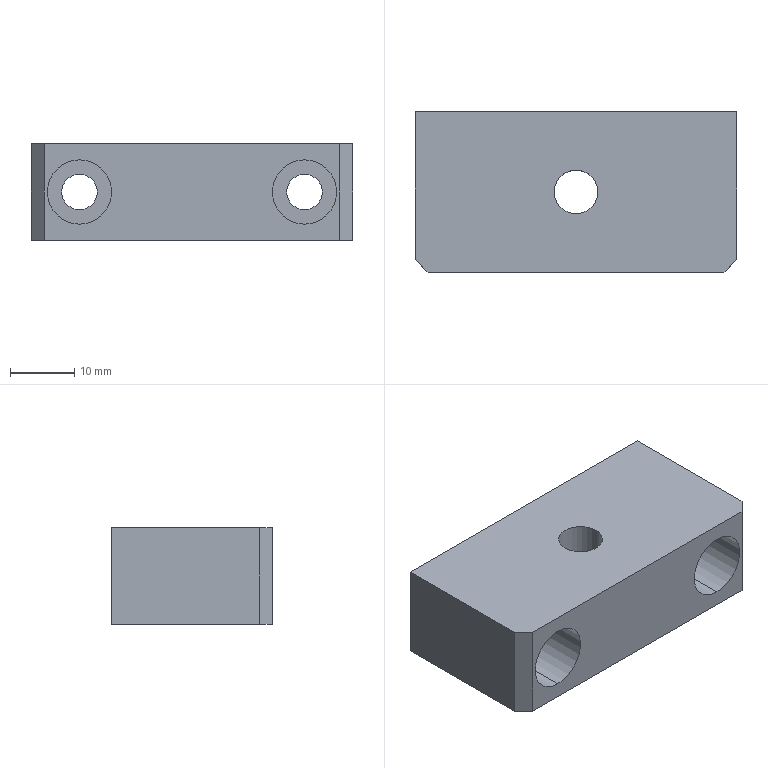Part | SolidWorks | features HoleWzd 2, Chamfer 1, Extrusion 1 | 1 solid | 20 faces | box 50 x 25 x 15 mm | volume 15237 mm3 | cylinder 10 | plane 10 | commonest cylinder face diameters 5.5 x4 10 x4 6.8 x2
STEP:
#1=CARTESIAN_POINT('',(-3.4,0.,0.));
#2=VERTEX_POINT('',#1);
#3=CARTESIAN_POINT('',(3.4,0.,0.));
#4=VERTEX_POINT('',#3);
#5=CARTESIAN_POINT('',(0.,0.,0.));
#6=DIRECTION('',(0.,0.,1.));
#7=DIRECTION('',(1.,0.,0.));
#8=AXIS2_PLACEMENT_3D('',#5,#6,#7);
#9=CIRCLE('',#8,3.4);
#10=EDGE_CURVE('',#2,#4,#9,.T.);
#11=ORIENTED_EDGE('',*,*,#10,.F.);
#12=CARTESIAN_POINT('',(-3.4,0.,15.));
#13=VERTEX_POINT('',#12);
#14=CARTESIAN_POINT('',(-3.4,0.,15.));
#15=DIRECTION('',(0.,0.,1.));
#16=VECTOR('',#15,1000.);
#17=LINE('',#14,#16);
#18=EDGE_CURVE('',#2,#13,#17,.T.);
#19=ORIENTED_EDGE('',*,*,#18,.T.);
#20=CARTESIAN_POINT('',(3.4,0.,15.));
#21=VERTEX_POINT('',#20);
#22=CARTESIAN_POINT('',(0.,0.,15.));
#23=DIRECTION('',(0.,0.,1.));
#24=DIRECTION('',(1.,0.,0.));
#25=AXIS2_PLACEMENT_3D('',#22,#23,#24);
#26=CIRCLE('',#25,3.4);
#27=EDGE_CURVE('',#13,#21,#26,.T.);
#28=ORIENTED_EDGE('',*,*,#27,.T.);
#29=CARTESIAN_POINT('',(3.4,0.,15.));
#30=DIRECTION('',(0.,0.,1.));
#31=VECTOR('',#30,1000.);
#32=LINE('',#29,#31);
#33=EDGE_CURVE('',#4,#21,#32,.T.);
#34=ORIENTED_EDGE('',*,*,#33,.F.);
#35=EDGE_LOOP('',(#11,#19,#28,#34));
#36=FACE_OUTER_BOUND('',#35,.T.);
#37=CARTESIAN_POINT('',(0.,0.,15.));
#38=DIRECTION('',(0.,0.,1.));
#39=DIRECTION('',(1.,0.,0.));
#40=AXIS2_PLACEMENT_3D('',#37,#38,#39);
#41=CYLINDRICAL_SURFACE('',#40,3.4);
#42=ADVANCED_FACE('',(#36),#41,.F.);
#43=CARTESIAN_POINT('',(17.5,3.2,12.5));
#44=VERTEX_POINT('',#43);
#45=CARTESIAN_POINT('',(17.5,3.2,2.5));
#46=VERTEX_POINT('',#45);
#47=CARTESIAN_POINT('',(17.5,3.2,7.5));
#48=DIRECTION('',(0.,-1.,0.));
#49=DIRECTION('',(0.,0.,-1.));
#50=AXIS2_PLACEMENT_3D('',#47,#48,#49);
#51=CIRCLE('',#50,5.);
#52=EDGE_CURVE('',#44,#46,#51,.T.);
#53=ORIENTED_EDGE('',*,*,#52,.F.);
#54=CARTESIAN_POINT('',(17.5,-12.5,12.5));
#55=VERTEX_POINT('',#54);
#56=CARTESIAN_POINT('',(17.5,-12.5,12.5));
#57=DIRECTION('',(0.,-1.,0.));
#58=VECTOR('',#57,1000.);
#59=LINE('',#56,#58);
#60=EDGE_CURVE('',#44,#55,#59,.T.);
#61=ORIENTED_EDGE('',*,*,#60,.T.);
#62=CARTESIAN_POINT('',(17.5,-12.5,2.5));
#63=VERTEX_POINT('',#62);
#64=CARTESIAN_POINT('',(17.5,-12.5,7.5));
#65=DIRECTION('',(0.,-1.,0.));
#66=DIRECTION('',(0.,0.,-1.));
#67=AXIS2_PLACEMENT_3D('',#64,#65,#66);
#68=CIRCLE('',#67,5.);
#69=EDGE_CURVE('',#55,#63,#68,.T.);
#70=ORIENTED_EDGE('',*,*,#69,.T.);
#71=CARTESIAN_POINT('',(17.5,-12.5,2.5));
#72=DIRECTION('',(0.,-1.,0.));
#73=VECTOR('',#72,1000.);
#74=LINE('',#71,#73);
#75=EDGE_CURVE('',#46,#63,#74,.T.);
#76=ORIENTED_EDGE('',*,*,#75,.F.);
#77=EDGE_LOOP('',(#53,#61,#70,#76));
#78=FACE_OUTER_BOUND('',#77,.T.);
#79=CARTESIAN_POINT('',(17.5,-12.5,7.5));
#80=DIRECTION('',(0.,-1.,0.));
#81=DIRECTION('',(0.,0.,-1.));
#82=AXIS2_PLACEMENT_3D('',#79,#80,#81);
#83=CYLINDRICAL_SURFACE('',#82,5.);
#84=ADVANCED_FACE('',(#78),#83,.F.);
#85=CARTESIAN_POINT('',(17.5,12.5,10.25));
#86=VERTEX_POINT('',#85);
#87=CARTESIAN_POINT('',(17.5,12.5,4.75));
#88=VERTEX_POINT('',#87);
#89=CARTESIAN_POINT('',(17.5,12.5,7.5));
#90=DIRECTION('',(0.,-1.,0.));
#91=DIRECTION('',(0.,0.,-1.));
#92=AXIS2_PLACEMENT_3D('',#89,#90,#91);
#93=CIRCLE('',#92,2.75);
#94=EDGE_CURVE('',#86,#88,#93,.T.);
#95=ORIENTED_EDGE('',*,*,#94,.F.);
#96=CARTESIAN_POINT('',(17.5,3.2,10.25));
#97=VERTEX_POINT('',#96);
#98=CARTESIAN_POINT('',(17.5,-12.5,10.25));
#99=DIRECTION('',(0.,-1.,0.));
#100=VECTOR('',#99,1000.);
#101=LINE('',#98,#100);
#102=EDGE_CURVE('',#86,#97,#101,.T.);
#103=ORIENTED_EDGE('',*,*,#102,.T.);
#104=CARTESIAN_POINT('',(17.5,3.2,4.75));
#105=VERTEX_POINT('',#104);
#106=CARTESIAN_POINT('',(17.5,3.2,7.5));
#107=DIRECTION('',(0.,-1.,0.));
#108=DIRECTION('',(0.,0.,-1.));
#109=AXIS2_PLACEMENT_3D('',#106,#107,#108);
#110=CIRCLE('',#109,2.75);
#111=EDGE_CURVE('',#97,#105,#110,.T.);
#112=ORIENTED_EDGE('',*,*,#111,.T.);
#113=CARTESIAN_POINT('',(17.5,-12.5,4.75));
#114=DIRECTION('',(0.,-1.,0.));
#115=VECTOR('',#114,1000.);
#116=LINE('',#113,#115);
#117=EDGE_CURVE('',#88,#105,#116,.T.);
#118=ORIENTED_EDGE('',*,*,#117,.F.);
#119=EDGE_LOOP('',(#95,#103,#112,#118));
#120=FACE_OUTER_BOUND('',#119,.T.);
#121=CARTESIAN_POINT('',(17.5,-12.5,7.5));
#122=DIRECTION('',(0.,-1.,0.));
#123=DIRECTION('',(0.,0.,-1.));
#124=AXIS2_PLACEMENT_3D('',#121,#122,#123);
#125=CYLINDRICAL_SURFACE('',#124,2.75);
#126=ADVANCED_FACE('',(#120),#125,.F.);
#127=CARTESIAN_POINT('',(-17.5,3.2,12.5));
#128=VERTEX_POINT('',#127);
#129=CARTESIAN_POINT('',(-17.5,3.2,2.5));
#130=VERTEX_POINT('',#129);
#131=CARTESIAN_POINT('',(-17.5,3.2,7.5));
#132=DIRECTION('',(0.,-1.,0.));
#133=DIRECTION('',(0.,0.,-1.));
#134=AXIS2_PLACEMENT_3D('',#131,#132,#133);
#135=CIRCLE('',#134,5.);
#136=EDGE_CURVE('',#128,#130,#135,.T.);
#137=ORIENTED_EDGE('',*,*,#136,.F.);
#138=CARTESIAN_POINT('',(-17.5,-12.5,12.5));
#139=VERTEX_POINT('',#138);
#140=CARTESIAN_POINT('',(-17.5,-12.5,12.5));
#141=DIRECTION('',(0.,-1.,0.));
#142=VECTOR('',#141,1000.);
#143=LINE('',#140,#142);
#144=EDGE_CURVE('',#128,#139,#143,.T.);
#145=ORIENTED_EDGE('',*,*,#144,.T.);
#146=CARTESIAN_POINT('',(-17.5,-12.5,2.5));
#147=VERTEX_POINT('',#146);
#148=CARTESIAN_POINT('',(-17.5,-12.5,7.5));
#149=DIRECTION('',(0.,-1.,0.));
#150=DIRECTION('',(0.,0.,-1.));
#151=AXIS2_PLACEMENT_3D('',#148,#149,#150);
#152=CIRCLE('',#151,5.);
#153=EDGE_CURVE('',#139,#147,#152,.T.);
#154=ORIENTED_EDGE('',*,*,#153,.T.);
#155=CARTESIAN_POINT('',(-17.5,-12.5,2.5));
#156=DIRECTION('',(0.,-1.,0.));
#157=VECTOR('',#156,1000.);
#158=LINE('',#155,#157);
#159=EDGE_CURVE('',#130,#147,#158,.T.);
#160=ORIENTED_EDGE('',*,*,#159,.F.);
#161=EDGE_LOOP('',(#137,#145,#154,#160));
#162=FACE_OUTER_BOUND('',#161,.T.);
#163=CARTESIAN_POINT('',(-17.5,-12.5,7.5));
#164=DIRECTION('',(0.,-1.,0.));
#165=DIRECTION('',(0.,0.,-1.));
#166=AXIS2_PLACEMENT_3D('',#163,#164,#165);
#167=CYLINDRICAL_SURFACE('',#166,5.);
#168=ADVANCED_FACE('',(#162),#167,.F.);
#169=CARTESIAN_POINT('',(-17.5,12.5,10.25));
#170=VERTEX_POINT('',#169);
#171=CARTESIAN_POINT('',(-17.5,12.5,4.75));
#172=VERTEX_POINT('',#171);
#173=CARTESIAN_POINT('',(-17.5,12.5,7.5));
#174=DIRECTION('',(0.,-1.,0.));
#175=DIRECTION('',(0.,0.,-1.));
#176=AXIS2_PLACEMENT_3D('',#173,#174,#175);
#177=CIRCLE('',#176,2.75);
#178=EDGE_CURVE('',#170,#172,#177,.T.);
#179=ORIENTED_EDGE('',*,*,#178,.F.);
#180=CARTESIAN_POINT('',(-17.5,3.2,10.25));
#181=VERTEX_POINT('',#180);
#182=CARTESIAN_POINT('',(-17.5,-12.5,10.25));
#183=DIRECTION('',(0.,-1.,0.));
#184=VECTOR('',#183,1000.);
#185=LINE('',#182,#184);
#186=EDGE_CURVE('',#170,#181,#185,.T.);
#187=ORIENTED_EDGE('',*,*,#186,.T.);
#188=CARTESIAN_POINT('',(-17.5,3.2,4.75));
#189=VERTEX_POINT('',#188);
#190=CARTESIAN_POINT('',(-17.5,3.2,7.5));
#191=DIRECTION('',(0.,-1.,0.));
#192=DIRECTION('',(0.,0.,-1.));
#193=AXIS2_PLACEMENT_3D('',#190,#191,#192);
#194=CIRCLE('',#193,2.75);
#195=EDGE_CURVE('',#181,#189,#194,.T.);
#196=ORIENTED_EDGE('',*,*,#195,.T.);
#197=CARTESIAN_POINT('',(-17.5,-12.5,4.75));
#198=DIRECTION('',(0.,-1.,0.));
#199=VECTOR('',#198,1000.);
#200=LINE('',#197,#199);
#201=EDGE_CURVE('',#172,#189,#200,.T.);
#202=ORIENTED_EDGE('',*,*,#201,.F.);
#203=EDGE_LOOP('',(#179,#187,#196,#202));
#204=FACE_OUTER_BOUND('',#203,.T.);
#205=CARTESIAN_POINT('',(-17.5,-12.5,7.5));
#206=DIRECTION('',(0.,-1.,0.));
#207=DIRECTION('',(0.,0.,-1.));
#208=AXIS2_PLACEMENT_3D('',#205,#206,#207);
#209=CYLINDRICAL_SURFACE('',#208,2.75);
#210=ADVANCED_FACE('',(#204),#209,.F.);
#211=CARTESIAN_POINT('',(25.,-10.5,15.));
#212=VERTEX_POINT('',#211);
#213=CARTESIAN_POINT('',(25.,12.5,15.));
#214=VERTEX_POINT('',#213);
#215=CARTESIAN_POINT('',(25.,-12.5,15.));
#216=DIRECTION('',(0.,1.,0.));
#217=VECTOR('',#216,1000.);
#218=LINE('',#215,#217);
#219=EDGE_CURVE('',#212,#214,#218,.T.);
#220=ORIENTED_EDGE('',*,*,#219,.F.);
#221=CARTESIAN_POINT('',(25.,-10.5,0.));
#222=VERTEX_POINT('',#221);
#223=CARTESIAN_POINT('',(25.,-10.5,15.));
#224=DIRECTION('',(0.,0.,-1.));
#225=VECTOR('',#224,1000.);
#226=LINE('',#223,#225);
#227=EDGE_CURVE('',#212,#222,#226,.T.);
#228=ORIENTED_EDGE('',*,*,#227,.T.);
#229=CARTESIAN_POINT('',(25.,12.5,0.));
#230=VERTEX_POINT('',#229);
#231=CARTESIAN_POINT('',(25.,-12.5,0.));
#232=DIRECTION('',(0.,1.,0.));
#233=VECTOR('',#232,1000.);
#234=LINE('',#231,#233);
#235=EDGE_CURVE('',#222,#230,#234,.T.);
#236=ORIENTED_EDGE('',*,*,#235,.T.);
#237=CARTESIAN_POINT('',(25.,12.5,15.));
#238=DIRECTION('',(0.,0.,-1.));
#239=VECTOR('',#238,1000.);
#240=LINE('',#237,#239);
#241=EDGE_CURVE('',#214,#230,#240,.T.);
#242=ORIENTED_EDGE('',*,*,#241,.F.);
#243=EDGE_LOOP('',(#220,#228,#236,#242));
#244=FACE_OUTER_BOUND('',#243,.T.);
#245=CARTESIAN_POINT('',(25.,-12.5,15.));
#246=DIRECTION('',(-1.,0.,0.));
#247=DIRECTION('',(0.,0.,1.));
#248=AXIS2_PLACEMENT_3D('',#245,#246,#247);
#249=PLANE('',#248);
#250=ADVANCED_FACE('',(#244),#249,.F.);
#251=CARTESIAN_POINT('',(17.5,12.5,7.5));
#252=DIRECTION('',(0.,-1.,0.));
#253=DIRECTION('',(0.,0.,-1.));
#254=AXIS2_PLACEMENT_3D('',#251,#252,#253);
#255=CIRCLE('',#254,2.75);
#256=EDGE_CURVE('',#88,#86,#255,.T.);
#257=ORIENTED_EDGE('',*,*,#256,.T.);
#258=ORIENTED_EDGE('',*,*,#94,.T.);
#259=EDGE_LOOP('',(#257,#258));
#260=FACE_BOUND('',#259,.T.);
#261=CARTESIAN_POINT('',(-17.5,12.5,7.5));
#262=DIRECTION('',(0.,-1.,0.));
#263=DIRECTION('',(0.,0.,-1.));
#264=AXIS2_PLACEMENT_3D('',#261,#262,#263);
#265=CIRCLE('',#264,2.75);
#266=EDGE_CURVE('',#172,#170,#265,.T.);
#267=ORIENTED_EDGE('',*,*,#266,.T.);
#268=ORIENTED_EDGE('',*,*,#178,.T.);
#269=EDGE_LOOP('',(#267,#268));
#270=FACE_BOUND('',#269,.T.);
#271=CARTESIAN_POINT('',(-25.,12.5,0.));
#272=VERTEX_POINT('',#271);
#273=CARTESIAN_POINT('',(-25.,12.5,0.));
#274=DIRECTION('',(-1.,0.,0.));
#275=VECTOR('',#274,1000.);
#276=LINE('',#273,#275);
#277=EDGE_CURVE('',#230,#272,#276,.T.);
#278=ORIENTED_EDGE('',*,*,#277,.T.);
#279=CARTESIAN_POINT('',(-25.,12.5,15.));
#280=VERTEX_POINT('',#279);
#281=CARTESIAN_POINT('',(-25.,12.5,15.));
#282=DIRECTION('',(0.,0.,-1.));
#283=VECTOR('',#282,1000.);
#284=LINE('',#281,#283);
#285=EDGE_CURVE('',#280,#272,#284,.T.);
#286=ORIENTED_EDGE('',*,*,#285,.F.);
#287=CARTESIAN_POINT('',(-25.,12.5,15.));
#288=DIRECTION('',(-1.,0.,0.));
#289=VECTOR('',#288,1000.);
#290=LINE('',#287,#289);
#291=EDGE_CURVE('',#214,#280,#290,.T.);
#292=ORIENTED_EDGE('',*,*,#291,.F.);
#293=ORIENTED_EDGE('',*,*,#241,.T.);
#294=EDGE_LOOP('',(#278,#286,#292,#293));
#295=FACE_OUTER_BOUND('',#294,.T.);
#296=CARTESIAN_POINT('',(-25.,12.5,15.));
#297=DIRECTION('',(0.,-1.,0.));
#298=DIRECTION('',(0.,0.,-1.));
#299=AXIS2_PLACEMENT_3D('',#296,#297,#298);
#300=PLANE('',#299);
#301=ADVANCED_FACE('',(#260,#270,#295),#300,.F.);
#302=CARTESIAN_POINT('',(-25.,-10.5,0.));
#303=VERTEX_POINT('',#302);
#304=CARTESIAN_POINT('',(-25.,-12.5,0.));
#305=DIRECTION('',(0.,-1.,0.));
#306=VECTOR('',#305,1000.);
#307=LINE('',#304,#306);
#308=EDGE_CURVE('',#272,#303,#307,.T.);
#309=ORIENTED_EDGE('',*,*,#308,.T.);
#310=CARTESIAN_POINT('',(-25.,-10.5,15.));
#311=VERTEX_POINT('',#310);
#312=CARTESIAN_POINT('',(-25.,-10.5,15.));
#313=DIRECTION('',(0.,0.,1.));
#314=VECTOR('',#313,1000.);
#315=LINE('',#312,#314);
#316=EDGE_CURVE('',#303,#311,#315,.T.);
#317=ORIENTED_EDGE('',*,*,#316,.T.);
#318=CARTESIAN_POINT('',(-25.,-12.5,15.));
#319=DIRECTION('',(0.,-1.,0.));
#320=VECTOR('',#319,1000.);
#321=LINE('',#318,#320);
#322=EDGE_CURVE('',#280,#311,#321,.T.);
#323=ORIENTED_EDGE('',*,*,#322,.F.);
#324=ORIENTED_EDGE('',*,*,#285,.T.);
#325=EDGE_LOOP('',(#309,#317,#323,#324));
#326=FACE_OUTER_BOUND('',#325,.T.);
#327=CARTESIAN_POINT('',(-25.,-12.5,15.));
#328=DIRECTION('',(1.,0.,0.));
#329=DIRECTION('',(0.,0.,-1.));
#330=AXIS2_PLACEMENT_3D('',#327,#328,#329);
#331=PLANE('',#330);
#332=ADVANCED_FACE('',(#326),#331,.F.);
#333=CARTESIAN_POINT('',(17.5,-12.5,7.5));
#334=DIRECTION('',(0.,-1.,0.));
#335=DIRECTION('',(0.,0.,-1.));
#336=AXIS2_PLACEMENT_3D('',#333,#334,#335);
#337=CIRCLE('',#336,5.);
#338=EDGE_CURVE('',#63,#55,#337,.T.);
#339=ORIENTED_EDGE('',*,*,#338,.F.);
#340=ORIENTED_EDGE('',*,*,#69,.F.);
#341=EDGE_LOOP('',(#339,#340));
#342=FACE_BOUND('',#341,.T.);
#343=CARTESIAN_POINT('',(-17.5,-12.5,7.5));
#344=DIRECTION('',(0.,-1.,0.));
#345=DIRECTION('',(0.,0.,-1.));
#346=AXIS2_PLACEMENT_3D('',#343,#344,#345);
#347=CIRCLE('',#346,5.);
#348=EDGE_CURVE('',#147,#139,#347,.T.);
#349=ORIENTED_EDGE('',*,*,#348,.F.);
#350=ORIENTED_EDGE('',*,*,#153,.F.);
#351=EDGE_LOOP('',(#349,#350));
#352=FACE_BOUND('',#351,.T.);
#353=CARTESIAN_POINT('',(-23.,-12.5,0.));
#354=VERTEX_POINT('',#353);
#355=CARTESIAN_POINT('',(23.,-12.5,0.));
#356=VERTEX_POINT('',#355);
#357=CARTESIAN_POINT('',(-25.,-12.5,0.));
#358=DIRECTION('',(1.,0.,0.));
#359=VECTOR('',#358,1000.);
#360=LINE('',#357,#359);
#361=EDGE_CURVE('',#354,#356,#360,.T.);
#362=ORIENTED_EDGE('',*,*,#361,.T.);
#363=CARTESIAN_POINT('',(23.,-12.5,15.));
#364=VERTEX_POINT('',#363);
#365=CARTESIAN_POINT('',(23.,-12.5,15.));
#366=DIRECTION('',(0.,0.,1.));
#367=VECTOR('',#366,1000.);
#368=LINE('',#365,#367);
#369=EDGE_CURVE('',#356,#364,#368,.T.);
#370=ORIENTED_EDGE('',*,*,#369,.T.);
#371=CARTESIAN_POINT('',(-23.,-12.5,15.));
#372=VERTEX_POINT('',#371);
#373=CARTESIAN_POINT('',(-25.,-12.5,15.));
#374=DIRECTION('',(1.,0.,0.));
#375=VECTOR('',#374,1000.);
#376=LINE('',#373,#375);
#377=EDGE_CURVE('',#372,#364,#376,.T.);
#378=ORIENTED_EDGE('',*,*,#377,.F.);
#379=CARTESIAN_POINT('',(-23.,-12.5,15.));
#380=DIRECTION('',(0.,0.,-1.));
#381=VECTOR('',#380,1000.);
#382=LINE('',#379,#381);
#383=EDGE_CURVE('',#372,#354,#382,.T.);
#384=ORIENTED_EDGE('',*,*,#383,.T.);
#385=EDGE_LOOP('',(#362,#370,#378,#384));
#386=FACE_OUTER_BOUND('',#385,.T.);
#387=CARTESIAN_POINT('',(-25.,-12.5,15.));
#388=DIRECTION('',(0.,1.,0.));
#389=DIRECTION('',(0.,0.,1.));
#390=AXIS2_PLACEMENT_3D('',#387,#388,#389);
#391=PLANE('',#390);
#392=ADVANCED_FACE('',(#342,#352,#386),#391,.F.);
#393=CARTESIAN_POINT('',(0.,0.,15.));
#394=DIRECTION('',(0.,0.,1.));
#395=DIRECTION('',(1.,0.,0.));
#396=AXIS2_PLACEMENT_3D('',#393,#394,#395);
#397=CIRCLE('',#396,3.4);
#398=EDGE_CURVE('',#21,#13,#397,.T.);
#399=ORIENTED_EDGE('',*,*,#398,.F.);
#400=ORIENTED_EDGE('',*,*,#27,.F.);
#401=EDGE_LOOP('',(#399,#400));
#402=FACE_BOUND('',#401,.T.);
#403=ORIENTED_EDGE('',*,*,#377,.T.);
#404=CARTESIAN_POINT('',(25.,-10.5,15.));
#405=DIRECTION('',(0.7071,0.7071,0.));
#406=VECTOR('',#405,1000.);
#407=LINE('',#404,#406);
#408=EDGE_CURVE('',#364,#212,#407,.T.);
#409=ORIENTED_EDGE('',*,*,#408,.T.);
#410=ORIENTED_EDGE('',*,*,#219,.T.);
#411=ORIENTED_EDGE('',*,*,#291,.T.);
#412=ORIENTED_EDGE('',*,*,#322,.T.);
#413=CARTESIAN_POINT('',(-23.,-12.5,15.));
#414=DIRECTION('',(0.7071,-0.7071,0.));
#415=VECTOR('',#414,1000.);
#416=LINE('',#413,#415);
#417=EDGE_CURVE('',#311,#372,#416,.T.);
#418=ORIENTED_EDGE('',*,*,#417,.T.);
#419=EDGE_LOOP('',(#403,#409,#410,#411,#412,#418));
#420=FACE_OUTER_BOUND('',#419,.T.);
#421=CARTESIAN_POINT('',(0.,0.,15.));
#422=DIRECTION('',(0.,0.,-1.));
#423=DIRECTION('',(-1.,0.,0.));
#424=AXIS2_PLACEMENT_3D('',#421,#422,#423);
#425=PLANE('',#424);
#426=ADVANCED_FACE('',(#402,#420),#425,.F.);
#427=CARTESIAN_POINT('',(0.,0.,0.));
#428=DIRECTION('',(0.,0.,1.));
#429=DIRECTION('',(1.,0.,0.));
#430=AXIS2_PLACEMENT_3D('',#427,#428,#429);
#431=CIRCLE('',#430,3.4);
#432=EDGE_CURVE('',#4,#2,#431,.T.);
#433=ORIENTED_EDGE('',*,*,#432,.T.);
#434=ORIENTED_EDGE('',*,*,#10,.T.);
#435=EDGE_LOOP('',(#433,#434));
#436=FACE_BOUND('',#435,.T.);
#437=ORIENTED_EDGE('',*,*,#235,.F.);
#438=CARTESIAN_POINT('',(17.75,-17.75,0.));
#439=DIRECTION('',(-0.7071,-0.7071,0.));
#440=VECTOR('',#439,1000.);
#441=LINE('',#438,#440);
#442=EDGE_CURVE('',#222,#356,#441,.T.);
#443=ORIENTED_EDGE('',*,*,#442,.T.);
#444=ORIENTED_EDGE('',*,*,#361,.F.);
#445=CARTESIAN_POINT('',(-17.75,-17.75,0.));
#446=DIRECTION('',(-0.7071,0.7071,0.));
#447=VECTOR('',#446,1000.);
#448=LINE('',#445,#447);
#449=EDGE_CURVE('',#354,#303,#448,.T.);
#450=ORIENTED_EDGE('',*,*,#449,.T.);
#451=ORIENTED_EDGE('',*,*,#308,.F.);
#452=ORIENTED_EDGE('',*,*,#277,.F.);
#453=EDGE_LOOP('',(#437,#443,#444,#450,#451,#452));
#454=FACE_OUTER_BOUND('',#453,.T.);
#455=CARTESIAN_POINT('',(0.,0.,0.));
#456=DIRECTION('',(0.,0.,-1.));
#457=DIRECTION('',(-1.,0.,0.));
#458=AXIS2_PLACEMENT_3D('',#455,#456,#457);
#459=PLANE('',#458);
#460=ADVANCED_FACE('',(#436,#454),#459,.T.);
#461=ORIENTED_EDGE('',*,*,#408,.F.);
#462=ORIENTED_EDGE('',*,*,#369,.F.);
#463=ORIENTED_EDGE('',*,*,#442,.F.);
#464=ORIENTED_EDGE('',*,*,#227,.F.);
#465=EDGE_LOOP('',(#461,#462,#463,#464));
#466=FACE_OUTER_BOUND('',#465,.T.);
#467=CARTESIAN_POINT('',(25.,-10.5,15.));
#468=DIRECTION('',(-0.7071,0.7071,0.));
#469=DIRECTION('',(0.,0.,-1.));
#470=AXIS2_PLACEMENT_3D('',#467,#468,#469);
#471=PLANE('',#470);
#472=ADVANCED_FACE('',(#466),#471,.F.);
#473=ORIENTED_EDGE('',*,*,#417,.F.);
#474=ORIENTED_EDGE('',*,*,#316,.F.);
#475=ORIENTED_EDGE('',*,*,#449,.F.);
#476=ORIENTED_EDGE('',*,*,#383,.F.);
#477=EDGE_LOOP('',(#473,#474,#475,#476));
#478=FACE_OUTER_BOUND('',#477,.T.);
#479=CARTESIAN_POINT('',(-23.,-12.5,15.));
#480=DIRECTION('',(0.7071,0.7071,0.));
#481=DIRECTION('',(0.,0.,-1.));
#482=AXIS2_PLACEMENT_3D('',#479,#480,#481);
#483=PLANE('',#482);
#484=ADVANCED_FACE('',(#478),#483,.F.);
#485=ORIENTED_EDGE('',*,*,#186,.F.);
#486=ORIENTED_EDGE('',*,*,#266,.F.);
#487=ORIENTED_EDGE('',*,*,#201,.T.);
#488=CARTESIAN_POINT('',(-17.5,3.2,7.5));
#489=DIRECTION('',(0.,-1.,0.));
#490=DIRECTION('',(0.,0.,-1.));
#491=AXIS2_PLACEMENT_3D('',#488,#489,#490);
#492=CIRCLE('',#491,2.75);
#493=EDGE_CURVE('',#189,#181,#492,.T.);
#494=ORIENTED_EDGE('',*,*,#493,.T.);
#495=EDGE_LOOP('',(#485,#486,#487,#494));
#496=FACE_OUTER_BOUND('',#495,.T.);
#497=CARTESIAN_POINT('',(-17.5,-12.5,7.5));
#498=DIRECTION('',(0.,-1.,0.));
#499=DIRECTION('',(0.,0.,-1.));
#500=AXIS2_PLACEMENT_3D('',#497,#498,#499);
#501=CYLINDRICAL_SURFACE('',#500,2.75);
#502=ADVANCED_FACE('',(#496),#501,.F.);
#503=ORIENTED_EDGE('',*,*,#493,.F.);
#504=ORIENTED_EDGE('',*,*,#195,.F.);
#505=EDGE_LOOP('',(#503,#504));
#506=FACE_BOUND('',#505,.T.);
#507=CARTESIAN_POINT('',(-17.5,3.2,7.5));
#508=DIRECTION('',(0.,-1.,0.));
#509=DIRECTION('',(0.,0.,-1.));
#510=AXIS2_PLACEMENT_3D('',#507,#508,#509);
#511=CIRCLE('',#510,5.);
#512=EDGE_CURVE('',#130,#128,#511,.T.);
#513=ORIENTED_EDGE('',*,*,#512,.T.);
#514=ORIENTED_EDGE('',*,*,#136,.T.);
#515=EDGE_LOOP('',(#513,#514));
#516=FACE_OUTER_BOUND('',#515,.T.);
#517=CARTESIAN_POINT('',(-14.75,3.2,7.5));
#518=DIRECTION('',(0.,1.,0.));
#519=DIRECTION('',(0.,0.,1.));
#520=AXIS2_PLACEMENT_3D('',#517,#518,#519);
#521=PLANE('',#520);
#522=ADVANCED_FACE('',(#506,#516),#521,.F.);
#523=ORIENTED_EDGE('',*,*,#144,.F.);
#524=ORIENTED_EDGE('',*,*,#512,.F.);
#525=ORIENTED_EDGE('',*,*,#159,.T.);
#526=ORIENTED_EDGE('',*,*,#348,.T.);
#527=EDGE_LOOP('',(#523,#524,#525,#526));
#528=FACE_OUTER_BOUND('',#527,.T.);
#529=CARTESIAN_POINT('',(-17.5,-12.5,7.5));
#530=DIRECTION('',(0.,-1.,0.));
#531=DIRECTION('',(0.,0.,-1.));
#532=AXIS2_PLACEMENT_3D('',#529,#530,#531);
#533=CYLINDRICAL_SURFACE('',#532,5.);
#534=ADVANCED_FACE('',(#528),#533,.F.);
#535=ORIENTED_EDGE('',*,*,#102,.F.);
#536=ORIENTED_EDGE('',*,*,#256,.F.);
#537=ORIENTED_EDGE('',*,*,#117,.T.);
#538=CARTESIAN_POINT('',(17.5,3.2,7.5));
#539=DIRECTION('',(0.,-1.,0.));
#540=DIRECTION('',(0.,0.,-1.));
#541=AXIS2_PLACEMENT_3D('',#538,#539,#540);
#542=CIRCLE('',#541,2.75);
#543=EDGE_CURVE('',#105,#97,#542,.T.);
#544=ORIENTED_EDGE('',*,*,#543,.T.);
#545=EDGE_LOOP('',(#535,#536,#537,#544));
#546=FACE_OUTER_BOUND('',#545,.T.);
#547=CARTESIAN_POINT('',(17.5,-12.5,7.5));
#548=DIRECTION('',(0.,-1.,0.));
#549=DIRECTION('',(0.,0.,-1.));
#550=AXIS2_PLACEMENT_3D('',#547,#548,#549);
#551=CYLINDRICAL_SURFACE('',#550,2.75);
#552=ADVANCED_FACE('',(#546),#551,.F.);
#553=ORIENTED_EDGE('',*,*,#543,.F.);
#554=ORIENTED_EDGE('',*,*,#111,.F.);
#555=EDGE_LOOP('',(#553,#554));
#556=FACE_BOUND('',#555,.T.);
#557=CARTESIAN_POINT('',(17.5,3.2,7.5));
#558=DIRECTION('',(0.,-1.,0.));
#559=DIRECTION('',(0.,0.,-1.));
#560=AXIS2_PLACEMENT_3D('',#557,#558,#559);
#561=CIRCLE('',#560,5.);
#562=EDGE_CURVE('',#46,#44,#561,.T.);
#563=ORIENTED_EDGE('',*,*,#562,.T.);
#564=ORIENTED_EDGE('',*,*,#52,.T.);
#565=EDGE_LOOP('',(#563,#564));
#566=FACE_OUTER_BOUND('',#565,.T.);
#567=CARTESIAN_POINT('',(20.25,3.2,7.5));
#568=DIRECTION('',(0.,1.,0.));
#569=DIRECTION('',(0.,0.,1.));
#570=AXIS2_PLACEMENT_3D('',#567,#568,#569);
#571=PLANE('',#570);
#572=ADVANCED_FACE('',(#556,#566),#571,.F.);
#573=ORIENTED_EDGE('',*,*,#60,.F.);
#574=ORIENTED_EDGE('',*,*,#562,.F.);
#575=ORIENTED_EDGE('',*,*,#75,.T.);
#576=ORIENTED_EDGE('',*,*,#338,.T.);
#577=EDGE_LOOP('',(#573,#574,#575,#576));
#578=FACE_OUTER_BOUND('',#577,.T.);
#579=CARTESIAN_POINT('',(17.5,-12.5,7.5));
#580=DIRECTION('',(0.,-1.,0.));
#581=DIRECTION('',(0.,0.,-1.));
#582=AXIS2_PLACEMENT_3D('',#579,#580,#581);
#583=CYLINDRICAL_SURFACE('',#582,5.);
#584=ADVANCED_FACE('',(#578),#583,.F.);
#585=ORIENTED_EDGE('',*,*,#18,.F.);
#586=ORIENTED_EDGE('',*,*,#432,.F.);
#587=ORIENTED_EDGE('',*,*,#33,.T.);
#588=ORIENTED_EDGE('',*,*,#398,.T.);
#589=EDGE_LOOP('',(#585,#586,#587,#588));
#590=FACE_OUTER_BOUND('',#589,.T.);
#591=CARTESIAN_POINT('',(0.,0.,15.));
#592=DIRECTION('',(0.,0.,1.));
#593=DIRECTION('',(1.,0.,0.));
#594=AXIS2_PLACEMENT_3D('',#591,#592,#593);
#595=CYLINDRICAL_SURFACE('',#594,3.4);
#596=ADVANCED_FACE('',(#590),#595,.F.);
#597=CLOSED_SHELL('',(#42,#84,#126,#168,#210,#250,#301,#332,#392,#426,#460,#472,#484,#502,#522,#534,#552,#572,#584,#596));
#598=MANIFOLD_SOLID_BREP('',#597);
#599=CARTESIAN_POINT('',(0.,0.,0.));
#600=DIRECTION('',(0.,0.,1.));
#601=DIRECTION('',(1.,0.,0.));
#602=AXIS2_PLACEMENT_3D('',#599,#600,#601);
#603=(LENGTH_UNIT()NAMED_UNIT(*)SI_UNIT(.MILLI.,.METRE.));
#604=UNCERTAINTY_MEASURE_WITH_UNIT(LENGTH_MEASURE(0.00001),#603,'','');
#605=(NAMED_UNIT(*)PLANE_ANGLE_UNIT()SI_UNIT($,.RADIAN.));
#606=(NAMED_UNIT(*)SI_UNIT($,.STERADIAN.)SOLID_ANGLE_UNIT());
#607=(GEOMETRIC_REPRESENTATION_CONTEXT(3)GLOBAL_UNCERTAINTY_ASSIGNED_CONTEXT((#604))GLOBAL_UNIT_ASSIGNED_CONTEXT((#603,#605,#606))REPRESENTATION_CONTEXT('',''));
#608=ADVANCED_BREP_SHAPE_REPRESENTATION('',(#598,#602),#607);